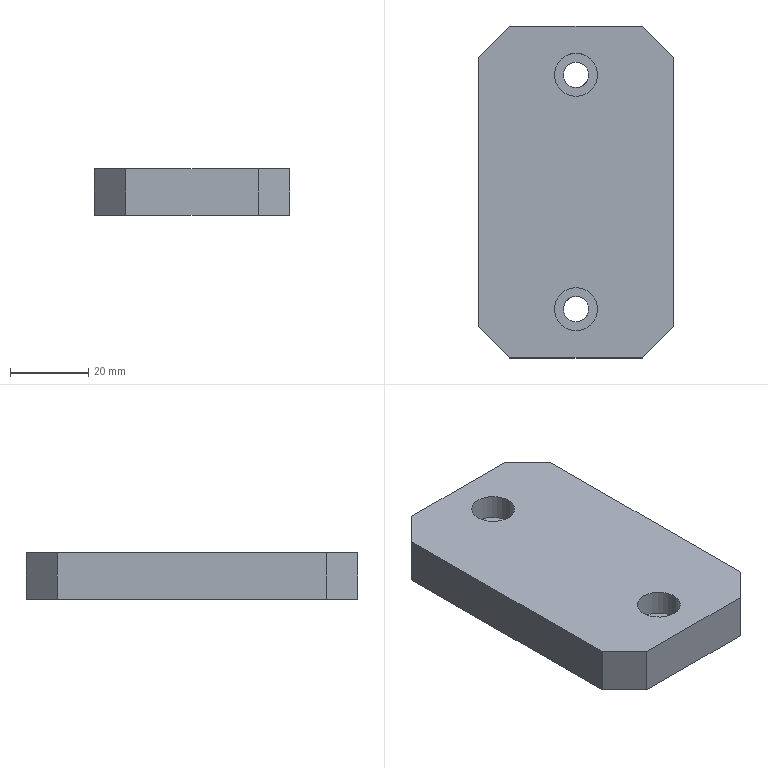Part | STEP file | P011002NM02-000 | 1 solid | 16 faces | box 50 x 85 x 12 mm | volume 47864 mm3 | plane 12 | cylinder 4 | commonest cylinder face diameters 6.5 x2 11 x2
STEP:
#1=CARTESIAN_POINT('',(0.,0.,0.));
#2=DIRECTION('',(0.,0.,1.));
#3=DIRECTION('',(1.,0.,0.));
#4=AXIS2_PLACEMENT_3D('',#1,#2,#3);
#5=CARTESIAN_POINT('',(227.,150.,9.));
#6=VERTEX_POINT('',#5);
#7=CARTESIAN_POINT('',(193.,150.,9.));
#8=VERTEX_POINT('',#7);
#9=CARTESIAN_POINT('',(210.,150.,9.));
#10=DIRECTION('',(-1.,0.,0.));
#11=VECTOR('',#10,1.);
#12=LINE('',#9,#11);
#13=CARTESIAN_POINT('',(210.,150.,6.));
#14=DIRECTION('',(0.,-1.,0.));
#15=DIRECTION('',(0.,0.,1.));
#16=AXIS2_PLACEMENT_3D('',#13,#14,#15);
#17=PLANE('',#16);
#18=CARTESIAN_POINT('',(3.,0.));
#19=DIRECTION('',(0.,1.));
#20=VECTOR('',#19,1.);
#21=LINE('',#18,#20);
#22=(GEOMETRIC_REPRESENTATION_CONTEXT(2)PARAMETRIC_REPRESENTATION_CONTEXT()REPRESENTATION_CONTEXT('',''));
#23=DEFINITIONAL_REPRESENTATION('',(#21),#22);
#24=PCURVE('',#17,#23);
#25=CARTESIAN_POINT('',(178.,-325.,9.));
#26=DIRECTION('',(0.,0.,1.));
#27=DIRECTION('',(1.,0.,0.));
#28=AXIS2_PLACEMENT_3D('',#25,#26,#27);
#29=PLANE('',#28);
#30=CARTESIAN_POINT('',(32.,475.));
#31=DIRECTION('',(-1.,0.));
#32=VECTOR('',#31,1.);
#33=LINE('',#30,#32);
#34=(GEOMETRIC_REPRESENTATION_CONTEXT(2)PARAMETRIC_REPRESENTATION_CONTEXT()REPRESENTATION_CONTEXT('',''));
#35=DEFINITIONAL_REPRESENTATION('',(#33),#34);
#36=PCURVE('',#29,#35);
#37=SURFACE_CURVE('',#12,(#24,#36),.PCURVE_S1.);
#38=EDGE_CURVE('',#6,#8,#37,.T.);
#39=ORIENTED_EDGE('',*,*,#38,.F.);
#40=CARTESIAN_POINT('',(227.,150.,21.));
#41=VERTEX_POINT('',#40);
#42=CARTESIAN_POINT('',(227.,150.,6.));
#43=DIRECTION('',(0.,0.,1.));
#44=VECTOR('',#43,1.);
#45=LINE('',#42,#44);
#46=CARTESIAN_POINT('',(0.,-17.));
#47=DIRECTION('',(1.,0.));
#48=VECTOR('',#47,1.);
#49=LINE('',#46,#48);
#50=(GEOMETRIC_REPRESENTATION_CONTEXT(2)PARAMETRIC_REPRESENTATION_CONTEXT()REPRESENTATION_CONTEXT('',''));
#51=DEFINITIONAL_REPRESENTATION('',(#49),#50);
#52=PCURVE('',#17,#51);
#53=CARTESIAN_POINT('',(235.,158.,6.));
#54=DIRECTION('',(-0.7071,0.7071,0.));
#55=DIRECTION('',(-0.7071,-0.7071,0.));
#56=AXIS2_PLACEMENT_3D('',#53,#54,#55);
#57=PLANE('',#56);
#58=CARTESIAN_POINT('',(11.314,0.));
#59=DIRECTION('',(0.,1.));
#60=VECTOR('',#59,1.);
#61=LINE('',#58,#60);
#62=(GEOMETRIC_REPRESENTATION_CONTEXT(2)PARAMETRIC_REPRESENTATION_CONTEXT()REPRESENTATION_CONTEXT('',''));
#63=DEFINITIONAL_REPRESENTATION('',(#61),#62);
#64=PCURVE('',#57,#63);
#65=SURFACE_CURVE('',#45,(#52,#64),.PCURVE_S1.);
#66=EDGE_CURVE('',#6,#41,#65,.T.);
#67=ORIENTED_EDGE('',*,*,#66,.T.);
#68=CARTESIAN_POINT('',(193.,150.,21.));
#69=VERTEX_POINT('',#68);
#70=CARTESIAN_POINT('',(210.,150.,21.));
#71=DIRECTION('',(-1.,0.,0.));
#72=VECTOR('',#71,1.);
#73=LINE('',#70,#72);
#74=CARTESIAN_POINT('',(15.,0.));
#75=DIRECTION('',(0.,1.));
#76=VECTOR('',#75,1.);
#77=LINE('',#74,#76);
#78=(GEOMETRIC_REPRESENTATION_CONTEXT(2)PARAMETRIC_REPRESENTATION_CONTEXT()REPRESENTATION_CONTEXT('',''));
#79=DEFINITIONAL_REPRESENTATION('',(#77),#78);
#80=PCURVE('',#17,#79);
#81=CARTESIAN_POINT('',(217.5,195.,21.));
#82=DIRECTION('',(0.,0.,1.));
#83=DIRECTION('',(1.,0.,0.));
#84=AXIS2_PLACEMENT_3D('',#81,#82,#83);
#85=PLANE('',#84);
#86=CARTESIAN_POINT('',(-7.5,-45.));
#87=DIRECTION('',(-1.,0.));
#88=VECTOR('',#87,1.);
#89=LINE('',#86,#88);
#90=(GEOMETRIC_REPRESENTATION_CONTEXT(2)PARAMETRIC_REPRESENTATION_CONTEXT()REPRESENTATION_CONTEXT('',''));
#91=DEFINITIONAL_REPRESENTATION('',(#89),#90);
#92=PCURVE('',#85,#91);
#93=SURFACE_CURVE('',#73,(#80,#92),.PCURVE_S1.);
#94=EDGE_CURVE('',#41,#69,#93,.T.);
#95=ORIENTED_EDGE('',*,*,#94,.T.);
#96=CARTESIAN_POINT('',(193.,150.,6.));
#97=DIRECTION('',(0.,0.,-1.));
#98=VECTOR('',#97,1.);
#99=LINE('',#96,#98);
#100=CARTESIAN_POINT('',(0.,17.));
#101=DIRECTION('',(-1.,0.));
#102=VECTOR('',#101,1.);
#103=LINE('',#100,#102);
#104=(GEOMETRIC_REPRESENTATION_CONTEXT(2)PARAMETRIC_REPRESENTATION_CONTEXT()REPRESENTATION_CONTEXT('',''));
#105=DEFINITIONAL_REPRESENTATION('',(#103),#104);
#106=PCURVE('',#17,#105);
#107=CARTESIAN_POINT('',(193.,150.,6.));
#108=DIRECTION('',(0.7071,0.7071,0.));
#109=DIRECTION('',(-0.7071,0.7071,0.));
#110=AXIS2_PLACEMENT_3D('',#107,#108,#109);
#111=PLANE('',#110);
#112=CARTESIAN_POINT('',(0.,0.));
#113=DIRECTION('',(0.,-1.));
#114=VECTOR('',#113,1.);
#115=LINE('',#112,#114);
#116=(GEOMETRIC_REPRESENTATION_CONTEXT(2)PARAMETRIC_REPRESENTATION_CONTEXT()REPRESENTATION_CONTEXT('',''));
#117=DEFINITIONAL_REPRESENTATION('',(#115),#116);
#118=PCURVE('',#111,#117);
#119=SURFACE_CURVE('',#99,(#106,#118),.PCURVE_S1.);
#120=EDGE_CURVE('',#69,#8,#119,.T.);
#121=ORIENTED_EDGE('',*,*,#120,.T.);
#122=EDGE_LOOP('',(#39,#67,#95,#121));
#123=FACE_BOUND('',#122,.T.);
#124=ADVANCED_FACE('',(#123),#17,.T.);
#125=CARTESIAN_POINT('',(235.,227.,9.));
#126=VERTEX_POINT('',#125);
#127=CARTESIAN_POINT('',(235.,158.,9.));
#128=VERTEX_POINT('',#127);
#129=CARTESIAN_POINT('',(235.,192.5,9.));
#130=DIRECTION('',(0.,-1.,0.));
#131=VECTOR('',#130,1.);
#132=LINE('',#129,#131);
#133=CARTESIAN_POINT('',(235.,192.5,6.));
#134=DIRECTION('',(1.,0.,0.));
#135=DIRECTION('',(0.,0.,-1.));
#136=AXIS2_PLACEMENT_3D('',#133,#134,#135);
#137=PLANE('',#136);
#138=CARTESIAN_POINT('',(-3.,0.));
#139=DIRECTION('',(0.,-1.));
#140=VECTOR('',#139,1.);
#141=LINE('',#138,#140);
#142=(GEOMETRIC_REPRESENTATION_CONTEXT(2)PARAMETRIC_REPRESENTATION_CONTEXT()REPRESENTATION_CONTEXT('',''));
#143=DEFINITIONAL_REPRESENTATION('',(#141),#142);
#144=PCURVE('',#137,#143);
#145=CARTESIAN_POINT('',(57.,517.5));
#146=DIRECTION('',(0.,-1.));
#147=VECTOR('',#146,1.);
#148=LINE('',#145,#147);
#149=(GEOMETRIC_REPRESENTATION_CONTEXT(2)PARAMETRIC_REPRESENTATION_CONTEXT()REPRESENTATION_CONTEXT('',''));
#150=DEFINITIONAL_REPRESENTATION('',(#148),#149);
#151=PCURVE('',#29,#150);
#152=SURFACE_CURVE('',#132,(#144,#151),.PCURVE_S1.);
#153=EDGE_CURVE('',#126,#128,#152,.T.);
#154=ORIENTED_EDGE('',*,*,#153,.F.);
#155=CARTESIAN_POINT('',(235.,227.,21.));
#156=VERTEX_POINT('',#155);
#157=CARTESIAN_POINT('',(235.,227.,6.));
#158=DIRECTION('',(0.,0.,1.));
#159=VECTOR('',#158,1.);
#160=LINE('',#157,#159);
#161=CARTESIAN_POINT('',(0.,34.5));
#162=DIRECTION('',(-1.,0.));
#163=VECTOR('',#162,1.);
#164=LINE('',#161,#163);
#165=(GEOMETRIC_REPRESENTATION_CONTEXT(2)PARAMETRIC_REPRESENTATION_CONTEXT()REPRESENTATION_CONTEXT('',''));
#166=DEFINITIONAL_REPRESENTATION('',(#164),#165);
#167=PCURVE('',#137,#166);
#168=CARTESIAN_POINT('',(227.,235.,6.));
#169=DIRECTION('',(-0.7071,-0.7071,0.));
#170=DIRECTION('',(0.7071,-0.7071,0.));
#171=AXIS2_PLACEMENT_3D('',#168,#169,#170);
#172=PLANE('',#171);
#173=CARTESIAN_POINT('',(11.314,0.));
#174=DIRECTION('',(0.,1.));
#175=VECTOR('',#174,1.);
#176=LINE('',#173,#175);
#177=(GEOMETRIC_REPRESENTATION_CONTEXT(2)PARAMETRIC_REPRESENTATION_CONTEXT()REPRESENTATION_CONTEXT('',''));
#178=DEFINITIONAL_REPRESENTATION('',(#176),#177);
#179=PCURVE('',#172,#178);
#180=SURFACE_CURVE('',#160,(#167,#179),.PCURVE_S1.);
#181=EDGE_CURVE('',#126,#156,#180,.T.);
#182=ORIENTED_EDGE('',*,*,#181,.T.);
#183=CARTESIAN_POINT('',(235.,158.,21.));
#184=VERTEX_POINT('',#183);
#185=CARTESIAN_POINT('',(235.,192.5,21.));
#186=DIRECTION('',(0.,-1.,0.));
#187=VECTOR('',#186,1.);
#188=LINE('',#185,#187);
#189=CARTESIAN_POINT('',(-15.,0.));
#190=DIRECTION('',(0.,-1.));
#191=VECTOR('',#190,1.);
#192=LINE('',#189,#191);
#193=(GEOMETRIC_REPRESENTATION_CONTEXT(2)PARAMETRIC_REPRESENTATION_CONTEXT()REPRESENTATION_CONTEXT('',''));
#194=DEFINITIONAL_REPRESENTATION('',(#192),#193);
#195=PCURVE('',#137,#194);
#196=CARTESIAN_POINT('',(17.5,-2.5));
#197=DIRECTION('',(0.,-1.));
#198=VECTOR('',#197,1.);
#199=LINE('',#196,#198);
#200=(GEOMETRIC_REPRESENTATION_CONTEXT(2)PARAMETRIC_REPRESENTATION_CONTEXT()REPRESENTATION_CONTEXT('',''));
#201=DEFINITIONAL_REPRESENTATION('',(#199),#200);
#202=PCURVE('',#85,#201);
#203=SURFACE_CURVE('',#188,(#195,#202),.PCURVE_S1.);
#204=EDGE_CURVE('',#156,#184,#203,.T.);
#205=ORIENTED_EDGE('',*,*,#204,.T.);
#206=CARTESIAN_POINT('',(235.,158.,6.));
#207=DIRECTION('',(0.,0.,-1.));
#208=VECTOR('',#207,1.);
#209=LINE('',#206,#208);
#210=CARTESIAN_POINT('',(0.,-34.5));
#211=DIRECTION('',(1.,0.));
#212=VECTOR('',#211,1.);
#213=LINE('',#210,#212);
#214=(GEOMETRIC_REPRESENTATION_CONTEXT(2)PARAMETRIC_REPRESENTATION_CONTEXT()REPRESENTATION_CONTEXT('',''));
#215=DEFINITIONAL_REPRESENTATION('',(#213),#214);
#216=PCURVE('',#137,#215);
#217=CARTESIAN_POINT('',(0.,0.));
#218=DIRECTION('',(0.,-1.));
#219=VECTOR('',#218,1.);
#220=LINE('',#217,#219);
#221=(GEOMETRIC_REPRESENTATION_CONTEXT(2)PARAMETRIC_REPRESENTATION_CONTEXT()REPRESENTATION_CONTEXT('',''));
#222=DEFINITIONAL_REPRESENTATION('',(#220),#221);
#223=PCURVE('',#57,#222);
#224=SURFACE_CURVE('',#209,(#216,#223),.PCURVE_S1.);
#225=EDGE_CURVE('',#184,#128,#224,.T.);
#226=ORIENTED_EDGE('',*,*,#225,.T.);
#227=EDGE_LOOP('',(#154,#182,#205,#226));
#228=FACE_BOUND('',#227,.T.);
#229=ADVANCED_FACE('',(#228),#137,.T.);
#230=CARTESIAN_POINT('',(193.,235.,9.));
#231=VERTEX_POINT('',#230);
#232=CARTESIAN_POINT('',(227.,235.,9.));
#233=VERTEX_POINT('',#232);
#234=CARTESIAN_POINT('',(210.,235.,9.));
#235=DIRECTION('',(1.,0.,0.));
#236=VECTOR('',#235,1.);
#237=LINE('',#234,#236);
#238=CARTESIAN_POINT('',(210.,235.,6.));
#239=DIRECTION('',(0.,1.,0.));
#240=DIRECTION('',(0.,0.,-1.));
#241=AXIS2_PLACEMENT_3D('',#238,#239,#240);
#242=PLANE('',#241);
#243=CARTESIAN_POINT('',(-3.,0.));
#244=DIRECTION('',(0.,-1.));
#245=VECTOR('',#244,1.);
#246=LINE('',#243,#245);
#247=(GEOMETRIC_REPRESENTATION_CONTEXT(2)PARAMETRIC_REPRESENTATION_CONTEXT()REPRESENTATION_CONTEXT('',''));
#248=DEFINITIONAL_REPRESENTATION('',(#246),#247);
#249=PCURVE('',#242,#248);
#250=CARTESIAN_POINT('',(32.,560.));
#251=DIRECTION('',(1.,0.));
#252=VECTOR('',#251,1.);
#253=LINE('',#250,#252);
#254=(GEOMETRIC_REPRESENTATION_CONTEXT(2)PARAMETRIC_REPRESENTATION_CONTEXT()REPRESENTATION_CONTEXT('',''));
#255=DEFINITIONAL_REPRESENTATION('',(#253),#254);
#256=PCURVE('',#29,#255);
#257=SURFACE_CURVE('',#237,(#249,#256),.PCURVE_S1.);
#258=EDGE_CURVE('',#231,#233,#257,.T.);
#259=ORIENTED_EDGE('',*,*,#258,.F.);
#260=CARTESIAN_POINT('',(193.,235.,21.));
#261=VERTEX_POINT('',#260);
#262=CARTESIAN_POINT('',(193.,235.,6.));
#263=DIRECTION('',(0.,0.,1.));
#264=VECTOR('',#263,1.);
#265=LINE('',#262,#264);
#266=CARTESIAN_POINT('',(0.,17.));
#267=DIRECTION('',(-1.,0.));
#268=VECTOR('',#267,1.);
#269=LINE('',#266,#268);
#270=(GEOMETRIC_REPRESENTATION_CONTEXT(2)PARAMETRIC_REPRESENTATION_CONTEXT()REPRESENTATION_CONTEXT('',''));
#271=DEFINITIONAL_REPRESENTATION('',(#269),#270);
#272=PCURVE('',#242,#271);
#273=CARTESIAN_POINT('',(185.,227.,6.));
#274=DIRECTION('',(0.7071,-0.7071,0.));
#275=DIRECTION('',(0.7071,0.7071,0.));
#276=AXIS2_PLACEMENT_3D('',#273,#274,#275);
#277=PLANE('',#276);
#278=CARTESIAN_POINT('',(11.314,0.));
#279=DIRECTION('',(0.,1.));
#280=VECTOR('',#279,1.);
#281=LINE('',#278,#280);
#282=(GEOMETRIC_REPRESENTATION_CONTEXT(2)PARAMETRIC_REPRESENTATION_CONTEXT()REPRESENTATION_CONTEXT('',''));
#283=DEFINITIONAL_REPRESENTATION('',(#281),#282);
#284=PCURVE('',#277,#283);
#285=SURFACE_CURVE('',#265,(#272,#284),.PCURVE_S1.);
#286=EDGE_CURVE('',#231,#261,#285,.T.);
#287=ORIENTED_EDGE('',*,*,#286,.T.);
#288=CARTESIAN_POINT('',(227.,235.,21.));
#289=VERTEX_POINT('',#288);
#290=CARTESIAN_POINT('',(210.,235.,21.));
#291=DIRECTION('',(1.,0.,0.));
#292=VECTOR('',#291,1.);
#293=LINE('',#290,#292);
#294=CARTESIAN_POINT('',(-15.,0.));
#295=DIRECTION('',(0.,-1.));
#296=VECTOR('',#295,1.);
#297=LINE('',#294,#296);
#298=(GEOMETRIC_REPRESENTATION_CONTEXT(2)PARAMETRIC_REPRESENTATION_CONTEXT()REPRESENTATION_CONTEXT('',''));
#299=DEFINITIONAL_REPRESENTATION('',(#297),#298);
#300=PCURVE('',#242,#299);
#301=CARTESIAN_POINT('',(-7.5,40.));
#302=DIRECTION('',(1.,0.));
#303=VECTOR('',#302,1.);
#304=LINE('',#301,#303);
#305=(GEOMETRIC_REPRESENTATION_CONTEXT(2)PARAMETRIC_REPRESENTATION_CONTEXT()REPRESENTATION_CONTEXT('',''));
#306=DEFINITIONAL_REPRESENTATION('',(#304),#305);
#307=PCURVE('',#85,#306);
#308=SURFACE_CURVE('',#293,(#300,#307),.PCURVE_S1.);
#309=EDGE_CURVE('',#261,#289,#308,.T.);
#310=ORIENTED_EDGE('',*,*,#309,.T.);
#311=CARTESIAN_POINT('',(227.,235.,6.));
#312=DIRECTION('',(0.,0.,-1.));
#313=VECTOR('',#312,1.);
#314=LINE('',#311,#313);
#315=CARTESIAN_POINT('',(0.,-17.));
#316=DIRECTION('',(1.,0.));
#317=VECTOR('',#316,1.);
#318=LINE('',#315,#317);
#319=(GEOMETRIC_REPRESENTATION_CONTEXT(2)PARAMETRIC_REPRESENTATION_CONTEXT()REPRESENTATION_CONTEXT('',''));
#320=DEFINITIONAL_REPRESENTATION('',(#318),#319);
#321=PCURVE('',#242,#320);
#322=CARTESIAN_POINT('',(0.,0.));
#323=DIRECTION('',(0.,-1.));
#324=VECTOR('',#323,1.);
#325=LINE('',#322,#324);
#326=(GEOMETRIC_REPRESENTATION_CONTEXT(2)PARAMETRIC_REPRESENTATION_CONTEXT()REPRESENTATION_CONTEXT('',''));
#327=DEFINITIONAL_REPRESENTATION('',(#325),#326);
#328=PCURVE('',#172,#327);
#329=SURFACE_CURVE('',#314,(#321,#328),.PCURVE_S1.);
#330=EDGE_CURVE('',#289,#233,#329,.T.);
#331=ORIENTED_EDGE('',*,*,#330,.T.);
#332=EDGE_LOOP('',(#259,#287,#310,#331));
#333=FACE_BOUND('',#332,.T.);
#334=ADVANCED_FACE('',(#333),#242,.T.);
#335=CARTESIAN_POINT('',(210.,157.,21.));
#336=VERTEX_POINT('',#335);
#337=CARTESIAN_POINT('',(210.,162.5,21.));
#338=DIRECTION('',(0.,0.,1.));
#339=DIRECTION('',(0.,-1.,0.));
#340=AXIS2_PLACEMENT_3D('',#337,#338,#339);
#341=CIRCLE('',#340,5.5);
#342=CARTESIAN_POINT('',(-7.5,-32.5));
#343=DIRECTION('',(0.,-1.));
#344=AXIS2_PLACEMENT_2D('',#342,#343);
#345=CIRCLE('',#344,5.5);
#346=(GEOMETRIC_REPRESENTATION_CONTEXT(2)PARAMETRIC_REPRESENTATION_CONTEXT()REPRESENTATION_CONTEXT('',''));
#347=DEFINITIONAL_REPRESENTATION('',(#345),#346);
#348=PCURVE('',#85,#347);
#349=CARTESIAN_POINT('',(210.,162.5,22.));
#350=DIRECTION('',(0.,0.,1.));
#351=DIRECTION('',(0.,-1.,0.));
#352=AXIS2_PLACEMENT_3D('',#349,#350,#351);
#353=CYLINDRICAL_SURFACE('',#352,5.5);
#354=CARTESIAN_POINT('',(0.,-1.));
#355=DIRECTION('',(1.,0.));
#356=VECTOR('',#355,1.);
#357=LINE('',#354,#356);
#358=(GEOMETRIC_REPRESENTATION_CONTEXT(2)PARAMETRIC_REPRESENTATION_CONTEXT()REPRESENTATION_CONTEXT('',''));
#359=DEFINITIONAL_REPRESENTATION('',(#357),#358);
#360=PCURVE('',#353,#359);
#361=SURFACE_CURVE('',#341,(#348,#360),.PCURVE_S1.);
#362=EDGE_CURVE('',#336,#336,#361,.T.);
#363=ORIENTED_EDGE('',*,*,#362,.F.);
#364=EDGE_LOOP('',(#363));
#365=FACE_BOUND('',#364,.T.);
#366=CARTESIAN_POINT('',(210.,217.,21.));
#367=VERTEX_POINT('',#366);
#368=CARTESIAN_POINT('',(210.,222.5,21.));
#369=DIRECTION('',(0.,0.,1.));
#370=DIRECTION('',(0.,-1.,0.));
#371=AXIS2_PLACEMENT_3D('',#368,#369,#370);
#372=CIRCLE('',#371,5.5);
#373=CARTESIAN_POINT('',(-7.5,27.5));
#374=DIRECTION('',(0.,-1.));
#375=AXIS2_PLACEMENT_2D('',#373,#374);
#376=CIRCLE('',#375,5.5);
#377=(GEOMETRIC_REPRESENTATION_CONTEXT(2)PARAMETRIC_REPRESENTATION_CONTEXT()REPRESENTATION_CONTEXT('',''));
#378=DEFINITIONAL_REPRESENTATION('',(#376),#377);
#379=PCURVE('',#85,#378);
#380=CARTESIAN_POINT('',(210.,222.5,22.));
#381=DIRECTION('',(0.,0.,1.));
#382=DIRECTION('',(0.,-1.,0.));
#383=AXIS2_PLACEMENT_3D('',#380,#381,#382);
#384=CYLINDRICAL_SURFACE('',#383,5.5);
#385=CARTESIAN_POINT('',(0.,-1.));
#386=DIRECTION('',(1.,0.));
#387=VECTOR('',#386,1.);
#388=LINE('',#385,#387);
#389=(GEOMETRIC_REPRESENTATION_CONTEXT(2)PARAMETRIC_REPRESENTATION_CONTEXT()REPRESENTATION_CONTEXT('',''));
#390=DEFINITIONAL_REPRESENTATION('',(#388),#389);
#391=PCURVE('',#384,#390);
#392=SURFACE_CURVE('',#372,(#379,#391),.PCURVE_S1.);
#393=EDGE_CURVE('',#367,#367,#392,.T.);
#394=ORIENTED_EDGE('',*,*,#393,.F.);
#395=EDGE_LOOP('',(#394));
#396=FACE_BOUND('',#395,.T.);
#397=CARTESIAN_POINT('',(185.,158.,21.));
#398=VERTEX_POINT('',#397);
#399=CARTESIAN_POINT('',(185.,227.,21.));
#400=VERTEX_POINT('',#399);
#401=CARTESIAN_POINT('',(185.,192.5,21.));
#402=DIRECTION('',(0.,1.,0.));
#403=VECTOR('',#402,1.);
#404=LINE('',#401,#403);
#405=CARTESIAN_POINT('',(-32.5,-2.5));
#406=DIRECTION('',(0.,1.));
#407=VECTOR('',#406,1.);
#408=LINE('',#405,#407);
#409=(GEOMETRIC_REPRESENTATION_CONTEXT(2)PARAMETRIC_REPRESENTATION_CONTEXT()REPRESENTATION_CONTEXT('',''));
#410=DEFINITIONAL_REPRESENTATION('',(#408),#409);
#411=PCURVE('',#85,#410);
#412=CARTESIAN_POINT('',(185.,192.5,6.));
#413=DIRECTION('',(-1.,0.,0.));
#414=DIRECTION('',(0.,0.,1.));
#415=AXIS2_PLACEMENT_3D('',#412,#413,#414);
#416=PLANE('',#415);
#417=CARTESIAN_POINT('',(15.,0.));
#418=DIRECTION('',(0.,1.));
#419=VECTOR('',#418,1.);
#420=LINE('',#417,#419);
#421=(GEOMETRIC_REPRESENTATION_CONTEXT(2)PARAMETRIC_REPRESENTATION_CONTEXT()REPRESENTATION_CONTEXT('',''));
#422=DEFINITIONAL_REPRESENTATION('',(#420),#421);
#423=PCURVE('',#416,#422);
#424=SURFACE_CURVE('',#404,(#411,#423),.PCURVE_S1.);
#425=EDGE_CURVE('',#398,#400,#424,.T.);
#426=ORIENTED_EDGE('',*,*,#425,.F.);
#427=CARTESIAN_POINT('',(182.75,160.25,21.));
#428=DIRECTION('',(0.7071,-0.7071,0.));
#429=VECTOR('',#428,1.);
#430=LINE('',#427,#429);
#431=CARTESIAN_POINT('',(-34.75,-34.75));
#432=DIRECTION('',(0.7071,-0.7071));
#433=VECTOR('',#432,1.);
#434=LINE('',#431,#433);
#435=(GEOMETRIC_REPRESENTATION_CONTEXT(2)PARAMETRIC_REPRESENTATION_CONTEXT()REPRESENTATION_CONTEXT('',''));
#436=DEFINITIONAL_REPRESENTATION('',(#434),#435);
#437=PCURVE('',#85,#436);
#438=CARTESIAN_POINT('',(14.496,15.));
#439=DIRECTION('',(-1.,0.));
#440=VECTOR('',#439,1.);
#441=LINE('',#438,#440);
#442=(GEOMETRIC_REPRESENTATION_CONTEXT(2)PARAMETRIC_REPRESENTATION_CONTEXT()REPRESENTATION_CONTEXT('',''));
#443=DEFINITIONAL_REPRESENTATION('',(#441),#442);
#444=PCURVE('',#111,#443);
#445=SURFACE_CURVE('',#430,(#437,#444),.PCURVE_S1.);
#446=EDGE_CURVE('',#398,#69,#445,.T.);
#447=ORIENTED_EDGE('',*,*,#446,.T.);
#448=ORIENTED_EDGE('',*,*,#94,.F.);
#449=CARTESIAN_POINT('',(244.75,167.75,21.));
#450=DIRECTION('',(0.7071,0.7071,0.));
#451=VECTOR('',#450,1.);
#452=LINE('',#449,#451);
#453=CARTESIAN_POINT('',(27.25,-27.25));
#454=DIRECTION('',(0.7071,0.7071));
#455=VECTOR('',#454,1.);
#456=LINE('',#453,#455);
#457=(GEOMETRIC_REPRESENTATION_CONTEXT(2)PARAMETRIC_REPRESENTATION_CONTEXT()REPRESENTATION_CONTEXT('',''));
#458=DEFINITIONAL_REPRESENTATION('',(#456),#457);
#459=PCURVE('',#85,#458);
#460=CARTESIAN_POINT('',(-13.789,15.));
#461=DIRECTION('',(-1.,0.));
#462=VECTOR('',#461,1.);
#463=LINE('',#460,#462);
#464=(GEOMETRIC_REPRESENTATION_CONTEXT(2)PARAMETRIC_REPRESENTATION_CONTEXT()REPRESENTATION_CONTEXT('',''));
#465=DEFINITIONAL_REPRESENTATION('',(#463),#464);
#466=PCURVE('',#57,#465);
#467=SURFACE_CURVE('',#452,(#459,#466),.PCURVE_S1.);
#468=EDGE_CURVE('',#41,#184,#467,.T.);
#469=ORIENTED_EDGE('',*,*,#468,.T.);
#470=ORIENTED_EDGE('',*,*,#204,.F.);
#471=CARTESIAN_POINT('',(242.25,219.75,21.));
#472=DIRECTION('',(-0.7071,0.7071,0.));
#473=VECTOR('',#472,1.);
#474=LINE('',#471,#473);
#475=CARTESIAN_POINT('',(24.75,24.75));
#476=DIRECTION('',(-0.7071,0.7071));
#477=VECTOR('',#476,1.);
#478=LINE('',#475,#477);
#479=(GEOMETRIC_REPRESENTATION_CONTEXT(2)PARAMETRIC_REPRESENTATION_CONTEXT()REPRESENTATION_CONTEXT('',''));
#480=DEFINITIONAL_REPRESENTATION('',(#478),#479);
#481=PCURVE('',#85,#480);
#482=CARTESIAN_POINT('',(21.567,15.));
#483=DIRECTION('',(-1.,0.));
#484=VECTOR('',#483,1.);
#485=LINE('',#482,#484);
#486=(GEOMETRIC_REPRESENTATION_CONTEXT(2)PARAMETRIC_REPRESENTATION_CONTEXT()REPRESENTATION_CONTEXT('',''));
#487=DEFINITIONAL_REPRESENTATION('',(#485),#486);
#488=PCURVE('',#172,#487);
#489=SURFACE_CURVE('',#474,(#481,#488),.PCURVE_S1.);
#490=EDGE_CURVE('',#156,#289,#489,.T.);
#491=ORIENTED_EDGE('',*,*,#490,.T.);
#492=ORIENTED_EDGE('',*,*,#309,.F.);
#493=CARTESIAN_POINT('',(185.25,227.25,21.));
#494=DIRECTION('',(-0.7071,-0.7071,0.));
#495=VECTOR('',#494,1.);
#496=LINE('',#493,#495);
#497=CARTESIAN_POINT('',(-32.25,32.25));
#498=DIRECTION('',(-0.7071,-0.7071));
#499=VECTOR('',#498,1.);
#500=LINE('',#497,#499);
#501=(GEOMETRIC_REPRESENTATION_CONTEXT(2)PARAMETRIC_REPRESENTATION_CONTEXT()REPRESENTATION_CONTEXT('',''));
#502=DEFINITIONAL_REPRESENTATION('',(#500),#501);
#503=PCURVE('',#85,#502);
#504=CARTESIAN_POINT('',(0.3536,15.));
#505=DIRECTION('',(-1.,0.));
#506=VECTOR('',#505,1.);
#507=LINE('',#504,#506);
#508=(GEOMETRIC_REPRESENTATION_CONTEXT(2)PARAMETRIC_REPRESENTATION_CONTEXT()REPRESENTATION_CONTEXT('',''));
#509=DEFINITIONAL_REPRESENTATION('',(#507),#508);
#510=PCURVE('',#277,#509);
#511=SURFACE_CURVE('',#496,(#503,#510),.PCURVE_S1.);
#512=EDGE_CURVE('',#261,#400,#511,.T.);
#513=ORIENTED_EDGE('',*,*,#512,.T.);
#514=EDGE_LOOP('',(#426,#447,#448,#469,#470,#491,#492,#513));
#515=FACE_BOUND('',#514,.T.);
#516=ADVANCED_FACE('',(#365,#396,#515),#85,.T.);
#517=CARTESIAN_POINT('',(185.,158.,9.));
#518=VERTEX_POINT('',#517);
#519=CARTESIAN_POINT('',(185.,227.,9.));
#520=VERTEX_POINT('',#519);
#521=CARTESIAN_POINT('',(185.,192.5,9.));
#522=DIRECTION('',(0.,1.,0.));
#523=VECTOR('',#522,1.);
#524=LINE('',#521,#523);
#525=CARTESIAN_POINT('',(3.,0.));
#526=DIRECTION('',(0.,1.));
#527=VECTOR('',#526,1.);
#528=LINE('',#525,#527);
#529=(GEOMETRIC_REPRESENTATION_CONTEXT(2)PARAMETRIC_REPRESENTATION_CONTEXT()REPRESENTATION_CONTEXT('',''));
#530=DEFINITIONAL_REPRESENTATION('',(#528),#529);
#531=PCURVE('',#416,#530);
#532=CARTESIAN_POINT('',(7.,517.5));
#533=DIRECTION('',(0.,1.));
#534=VECTOR('',#533,1.);
#535=LINE('',#532,#534);
#536=(GEOMETRIC_REPRESENTATION_CONTEXT(2)PARAMETRIC_REPRESENTATION_CONTEXT()REPRESENTATION_CONTEXT('',''));
#537=DEFINITIONAL_REPRESENTATION('',(#535),#536);
#538=PCURVE('',#29,#537);
#539=SURFACE_CURVE('',#524,(#531,#538),.PCURVE_S1.);
#540=EDGE_CURVE('',#518,#520,#539,.T.);
#541=ORIENTED_EDGE('',*,*,#540,.F.);
#542=CARTESIAN_POINT('',(185.,158.,6.));
#543=DIRECTION('',(0.,0.,1.));
#544=VECTOR('',#543,1.);
#545=LINE('',#542,#544);
#546=CARTESIAN_POINT('',(0.,-34.5));
#547=DIRECTION('',(1.,0.));
#548=VECTOR('',#547,1.);
#549=LINE('',#546,#548);
#550=(GEOMETRIC_REPRESENTATION_CONTEXT(2)PARAMETRIC_REPRESENTATION_CONTEXT()REPRESENTATION_CONTEXT('',''));
#551=DEFINITIONAL_REPRESENTATION('',(#549),#550);
#552=PCURVE('',#416,#551);
#553=CARTESIAN_POINT('',(11.314,0.));
#554=DIRECTION('',(0.,1.));
#555=VECTOR('',#554,1.);
#556=LINE('',#553,#555);
#557=(GEOMETRIC_REPRESENTATION_CONTEXT(2)PARAMETRIC_REPRESENTATION_CONTEXT()REPRESENTATION_CONTEXT('',''));
#558=DEFINITIONAL_REPRESENTATION('',(#556),#557);
#559=PCURVE('',#111,#558);
#560=SURFACE_CURVE('',#545,(#552,#559),.PCURVE_S1.);
#561=EDGE_CURVE('',#518,#398,#560,.T.);
#562=ORIENTED_EDGE('',*,*,#561,.T.);
#563=ORIENTED_EDGE('',*,*,#425,.T.);
#564=CARTESIAN_POINT('',(185.,227.,6.));
#565=DIRECTION('',(0.,0.,-1.));
#566=VECTOR('',#565,1.);
#567=LINE('',#564,#566);
#568=CARTESIAN_POINT('',(0.,34.5));
#569=DIRECTION('',(-1.,0.));
#570=VECTOR('',#569,1.);
#571=LINE('',#568,#570);
#572=(GEOMETRIC_REPRESENTATION_CONTEXT(2)PARAMETRIC_REPRESENTATION_CONTEXT()REPRESENTATION_CONTEXT('',''));
#573=DEFINITIONAL_REPRESENTATION('',(#571),#572);
#574=PCURVE('',#416,#573);
#575=CARTESIAN_POINT('',(0.,0.));
#576=DIRECTION('',(0.,-1.));
#577=VECTOR('',#576,1.);
#578=LINE('',#575,#577);
#579=(GEOMETRIC_REPRESENTATION_CONTEXT(2)PARAMETRIC_REPRESENTATION_CONTEXT()REPRESENTATION_CONTEXT('',''));
#580=DEFINITIONAL_REPRESENTATION('',(#578),#579);
#581=PCURVE('',#277,#580);
#582=SURFACE_CURVE('',#567,(#574,#581),.PCURVE_S1.);
#583=EDGE_CURVE('',#400,#520,#582,.T.);
#584=ORIENTED_EDGE('',*,*,#583,.T.);
#585=EDGE_LOOP('',(#541,#562,#563,#584));
#586=FACE_BOUND('',#585,.T.);
#587=ADVANCED_FACE('',(#586),#416,.T.);
#588=CARTESIAN_POINT('',(193.,150.,9.));
#589=DIRECTION('',(-0.7071,0.7071,0.));
#590=VECTOR('',#589,1.);
#591=LINE('',#588,#590);
#592=CARTESIAN_POINT('',(0.,3.));
#593=DIRECTION('',(1.,0.));
#594=VECTOR('',#593,1.);
#595=LINE('',#592,#594);
#596=(GEOMETRIC_REPRESENTATION_CONTEXT(2)PARAMETRIC_REPRESENTATION_CONTEXT()REPRESENTATION_CONTEXT('',''));
#597=DEFINITIONAL_REPRESENTATION('',(#595),#596);
#598=PCURVE('',#111,#597);
#599=CARTESIAN_POINT('',(15.,475.));
#600=DIRECTION('',(-0.7071,0.7071));
#601=VECTOR('',#600,1.);
#602=LINE('',#599,#601);
#603=(GEOMETRIC_REPRESENTATION_CONTEXT(2)PARAMETRIC_REPRESENTATION_CONTEXT()REPRESENTATION_CONTEXT('',''));
#604=DEFINITIONAL_REPRESENTATION('',(#602),#603);
#605=PCURVE('',#29,#604);
#606=SURFACE_CURVE('',#591,(#598,#605),.PCURVE_S1.);
#607=EDGE_CURVE('',#8,#518,#606,.T.);
#608=ORIENTED_EDGE('',*,*,#607,.F.);
#609=ORIENTED_EDGE('',*,*,#120,.F.);
#610=ORIENTED_EDGE('',*,*,#446,.F.);
#611=ORIENTED_EDGE('',*,*,#561,.F.);
#612=EDGE_LOOP('',(#608,#609,#610,#611));
#613=FACE_BOUND('',#612,.T.);
#614=ADVANCED_FACE('',(#613),#111,.F.);
#615=CARTESIAN_POINT('',(227.,235.,9.));
#616=DIRECTION('',(0.7071,-0.7071,0.));
#617=VECTOR('',#616,1.);
#618=LINE('',#615,#617);
#619=CARTESIAN_POINT('',(0.,3.));
#620=DIRECTION('',(1.,0.));
#621=VECTOR('',#620,1.);
#622=LINE('',#619,#621);
#623=(GEOMETRIC_REPRESENTATION_CONTEXT(2)PARAMETRIC_REPRESENTATION_CONTEXT()REPRESENTATION_CONTEXT('',''));
#624=DEFINITIONAL_REPRESENTATION('',(#622),#623);
#625=PCURVE('',#172,#624);
#626=CARTESIAN_POINT('',(49.,560.));
#627=DIRECTION('',(0.7071,-0.7071));
#628=VECTOR('',#627,1.);
#629=LINE('',#626,#628);
#630=(GEOMETRIC_REPRESENTATION_CONTEXT(2)PARAMETRIC_REPRESENTATION_CONTEXT()REPRESENTATION_CONTEXT('',''));
#631=DEFINITIONAL_REPRESENTATION('',(#629),#630);
#632=PCURVE('',#29,#631);
#633=SURFACE_CURVE('',#618,(#625,#632),.PCURVE_S1.);
#634=EDGE_CURVE('',#233,#126,#633,.T.);
#635=ORIENTED_EDGE('',*,*,#634,.F.);
#636=ORIENTED_EDGE('',*,*,#330,.F.);
#637=ORIENTED_EDGE('',*,*,#490,.F.);
#638=ORIENTED_EDGE('',*,*,#181,.F.);
#639=EDGE_LOOP('',(#635,#636,#637,#638));
#640=FACE_BOUND('',#639,.T.);
#641=ADVANCED_FACE('',(#640),#172,.F.);
#642=CARTESIAN_POINT('',(235.,158.,9.));
#643=DIRECTION('',(-0.7071,-0.7071,0.));
#644=VECTOR('',#643,1.);
#645=LINE('',#642,#644);
#646=CARTESIAN_POINT('',(0.,3.));
#647=DIRECTION('',(1.,0.));
#648=VECTOR('',#647,1.);
#649=LINE('',#646,#648);
#650=(GEOMETRIC_REPRESENTATION_CONTEXT(2)PARAMETRIC_REPRESENTATION_CONTEXT()REPRESENTATION_CONTEXT('',''));
#651=DEFINITIONAL_REPRESENTATION('',(#649),#650);
#652=PCURVE('',#57,#651);
#653=CARTESIAN_POINT('',(57.,483.));
#654=DIRECTION('',(-0.7071,-0.7071));
#655=VECTOR('',#654,1.);
#656=LINE('',#653,#655);
#657=(GEOMETRIC_REPRESENTATION_CONTEXT(2)PARAMETRIC_REPRESENTATION_CONTEXT()REPRESENTATION_CONTEXT('',''));
#658=DEFINITIONAL_REPRESENTATION('',(#656),#657);
#659=PCURVE('',#29,#658);
#660=SURFACE_CURVE('',#645,(#652,#659),.PCURVE_S1.);
#661=EDGE_CURVE('',#128,#6,#660,.T.);
#662=ORIENTED_EDGE('',*,*,#661,.F.);
#663=ORIENTED_EDGE('',*,*,#225,.F.);
#664=ORIENTED_EDGE('',*,*,#468,.F.);
#665=ORIENTED_EDGE('',*,*,#66,.F.);
#666=EDGE_LOOP('',(#662,#663,#664,#665));
#667=FACE_BOUND('',#666,.T.);
#668=ADVANCED_FACE('',(#667),#57,.F.);
#669=CARTESIAN_POINT('',(185.,227.,9.));
#670=DIRECTION('',(0.7071,0.7071,0.));
#671=VECTOR('',#670,1.);
#672=LINE('',#669,#671);
#673=CARTESIAN_POINT('',(0.,3.));
#674=DIRECTION('',(1.,0.));
#675=VECTOR('',#674,1.);
#676=LINE('',#673,#675);
#677=(GEOMETRIC_REPRESENTATION_CONTEXT(2)PARAMETRIC_REPRESENTATION_CONTEXT()REPRESENTATION_CONTEXT('',''));
#678=DEFINITIONAL_REPRESENTATION('',(#676),#677);
#679=PCURVE('',#277,#678);
#680=CARTESIAN_POINT('',(7.,552.));
#681=DIRECTION('',(0.7071,0.7071));
#682=VECTOR('',#681,1.);
#683=LINE('',#680,#682);
#684=(GEOMETRIC_REPRESENTATION_CONTEXT(2)PARAMETRIC_REPRESENTATION_CONTEXT()REPRESENTATION_CONTEXT('',''));
#685=DEFINITIONAL_REPRESENTATION('',(#683),#684);
#686=PCURVE('',#29,#685);
#687=SURFACE_CURVE('',#672,(#679,#686),.PCURVE_S1.);
#688=EDGE_CURVE('',#520,#231,#687,.T.);
#689=ORIENTED_EDGE('',*,*,#688,.F.);
#690=ORIENTED_EDGE('',*,*,#583,.F.);
#691=ORIENTED_EDGE('',*,*,#512,.F.);
#692=ORIENTED_EDGE('',*,*,#286,.F.);
#693=EDGE_LOOP('',(#689,#690,#691,#692));
#694=FACE_BOUND('',#693,.T.);
#695=ADVANCED_FACE('',(#694),#277,.F.);
#696=CARTESIAN_POINT('',(213.25,162.5,9.));
#697=VERTEX_POINT('',#696);
#698=CARTESIAN_POINT('',(210.,159.25,9.));
#699=VERTEX_POINT('',#698);
#700=CARTESIAN_POINT('',(210.,162.5,9.));
#701=DIRECTION('',(0.,0.,1.));
#702=DIRECTION('',(1.,0.,0.));
#703=AXIS2_PLACEMENT_3D('',#700,#701,#702);
#704=CIRCLE('',#703,3.25);
#705=CARTESIAN_POINT('',(32.,487.5));
#706=DIRECTION('',(1.,0.));
#707=AXIS2_PLACEMENT_2D('',#705,#706);
#708=CIRCLE('',#707,3.25);
#709=(GEOMETRIC_REPRESENTATION_CONTEXT(2)PARAMETRIC_REPRESENTATION_CONTEXT()REPRESENTATION_CONTEXT('',''));
#710=DEFINITIONAL_REPRESENTATION('',(#708),#709);
#711=PCURVE('',#29,#710);
#712=CARTESIAN_POINT('',(210.,162.5,22.));
#713=DIRECTION('',(0.,0.,1.));
#714=DIRECTION('',(0.,-1.,0.));
#715=AXIS2_PLACEMENT_3D('',#712,#713,#714);
#716=CYLINDRICAL_SURFACE('',#715,3.25);
#717=CARTESIAN_POINT('',(1.571,-13.));
#718=DIRECTION('',(1.,0.));
#719=VECTOR('',#718,1.);
#720=LINE('',#717,#719);
#721=(GEOMETRIC_REPRESENTATION_CONTEXT(2)PARAMETRIC_REPRESENTATION_CONTEXT()REPRESENTATION_CONTEXT('',''));
#722=DEFINITIONAL_REPRESENTATION('',(#720),#721);
#723=PCURVE('',#716,#722);
#724=SURFACE_CURVE('',#704,(#711,#723),.PCURVE_S1.);
#725=EDGE_CURVE('',#697,#699,#724,.T.);
#726=ORIENTED_EDGE('',*,*,#725,.T.);
#727=CARTESIAN_POINT('',(210.,162.5,9.));
#728=DIRECTION('',(0.,0.,1.));
#729=DIRECTION('',(1.,0.,0.));
#730=AXIS2_PLACEMENT_3D('',#727,#728,#729);
#731=CIRCLE('',#730,3.25);
#732=CARTESIAN_POINT('',(32.,487.5));
#733=DIRECTION('',(1.,0.));
#734=AXIS2_PLACEMENT_2D('',#732,#733);
#735=CIRCLE('',#734,3.25);
#736=(GEOMETRIC_REPRESENTATION_CONTEXT(2)PARAMETRIC_REPRESENTATION_CONTEXT()REPRESENTATION_CONTEXT('',''));
#737=DEFINITIONAL_REPRESENTATION('',(#735),#736);
#738=PCURVE('',#29,#737);
#739=CARTESIAN_POINT('',(-4.712,-13.));
#740=DIRECTION('',(1.,0.));
#741=VECTOR('',#740,1.);
#742=LINE('',#739,#741);
#743=(GEOMETRIC_REPRESENTATION_CONTEXT(2)PARAMETRIC_REPRESENTATION_CONTEXT()REPRESENTATION_CONTEXT('',''));
#744=DEFINITIONAL_REPRESENTATION('',(#742),#743);
#745=PCURVE('',#716,#744);
#746=SURFACE_CURVE('',#731,(#738,#745),.PCURVE_S1.);
#747=EDGE_CURVE('',#699,#697,#746,.T.);
#748=ORIENTED_EDGE('',*,*,#747,.T.);
#749=EDGE_LOOP('',(#726,#748));
#750=FACE_BOUND('',#749,.T.);
#751=CARTESIAN_POINT('',(213.25,222.5,9.));
#752=VERTEX_POINT('',#751);
#753=CARTESIAN_POINT('',(210.,219.25,9.));
#754=VERTEX_POINT('',#753);
#755=CARTESIAN_POINT('',(210.,222.5,9.));
#756=DIRECTION('',(0.,0.,1.));
#757=DIRECTION('',(1.,0.,0.));
#758=AXIS2_PLACEMENT_3D('',#755,#756,#757);
#759=CIRCLE('',#758,3.25);
#760=CARTESIAN_POINT('',(32.,547.5));
#761=DIRECTION('',(1.,0.));
#762=AXIS2_PLACEMENT_2D('',#760,#761);
#763=CIRCLE('',#762,3.25);
#764=(GEOMETRIC_REPRESENTATION_CONTEXT(2)PARAMETRIC_REPRESENTATION_CONTEXT()REPRESENTATION_CONTEXT('',''));
#765=DEFINITIONAL_REPRESENTATION('',(#763),#764);
#766=PCURVE('',#29,#765);
#767=CARTESIAN_POINT('',(210.,222.5,22.));
#768=DIRECTION('',(0.,0.,1.));
#769=DIRECTION('',(0.,-1.,0.));
#770=AXIS2_PLACEMENT_3D('',#767,#768,#769);
#771=CYLINDRICAL_SURFACE('',#770,3.25);
#772=CARTESIAN_POINT('',(1.571,-13.));
#773=DIRECTION('',(1.,0.));
#774=VECTOR('',#773,1.);
#775=LINE('',#772,#774);
#776=(GEOMETRIC_REPRESENTATION_CONTEXT(2)PARAMETRIC_REPRESENTATION_CONTEXT()REPRESENTATION_CONTEXT('',''));
#777=DEFINITIONAL_REPRESENTATION('',(#775),#776);
#778=PCURVE('',#771,#777);
#779=SURFACE_CURVE('',#759,(#766,#778),.PCURVE_S1.);
#780=EDGE_CURVE('',#752,#754,#779,.T.);
#781=ORIENTED_EDGE('',*,*,#780,.T.);
#782=CARTESIAN_POINT('',(210.,222.5,9.));
#783=DIRECTION('',(0.,0.,1.));
#784=DIRECTION('',(1.,0.,0.));
#785=AXIS2_PLACEMENT_3D('',#782,#783,#784);
#786=CIRCLE('',#785,3.25);
#787=CARTESIAN_POINT('',(32.,547.5));
#788=DIRECTION('',(1.,0.));
#789=AXIS2_PLACEMENT_2D('',#787,#788);
#790=CIRCLE('',#789,3.25);
#791=(GEOMETRIC_REPRESENTATION_CONTEXT(2)PARAMETRIC_REPRESENTATION_CONTEXT()REPRESENTATION_CONTEXT('',''));
#792=DEFINITIONAL_REPRESENTATION('',(#790),#791);
#793=PCURVE('',#29,#792);
#794=CARTESIAN_POINT('',(-4.712,-13.));
#795=DIRECTION('',(1.,0.));
#796=VECTOR('',#795,1.);
#797=LINE('',#794,#796);
#798=(GEOMETRIC_REPRESENTATION_CONTEXT(2)PARAMETRIC_REPRESENTATION_CONTEXT()REPRESENTATION_CONTEXT('',''));
#799=DEFINITIONAL_REPRESENTATION('',(#797),#798);
#800=PCURVE('',#771,#799);
#801=SURFACE_CURVE('',#786,(#793,#800),.PCURVE_S1.);
#802=EDGE_CURVE('',#754,#752,#801,.T.);
#803=ORIENTED_EDGE('',*,*,#802,.T.);
#804=EDGE_LOOP('',(#781,#803));
#805=FACE_BOUND('',#804,.T.);
#806=ORIENTED_EDGE('',*,*,#661,.T.);
#807=ORIENTED_EDGE('',*,*,#38,.T.);
#808=ORIENTED_EDGE('',*,*,#607,.T.);
#809=ORIENTED_EDGE('',*,*,#540,.T.);
#810=ORIENTED_EDGE('',*,*,#688,.T.);
#811=ORIENTED_EDGE('',*,*,#258,.T.);
#812=ORIENTED_EDGE('',*,*,#634,.T.);
#813=ORIENTED_EDGE('',*,*,#153,.T.);
#814=EDGE_LOOP('',(#806,#807,#808,#809,#810,#811,#812,#813));
#815=FACE_BOUND('',#814,.T.);
#816=ADVANCED_FACE('',(#750,#805,#815),#29,.F.);
#817=CARTESIAN_POINT('',(210.,219.25,14.5));
#818=VERTEX_POINT('',#817);
#819=CARTESIAN_POINT('',(210.,222.5,14.5));
#820=DIRECTION('',(0.,0.,1.));
#821=DIRECTION('',(0.,-1.,0.));
#822=AXIS2_PLACEMENT_3D('',#819,#820,#821);
#823=CIRCLE('',#822,3.25);
#824=CARTESIAN_POINT('',(0.,-7.5));
#825=DIRECTION('',(1.,0.));
#826=VECTOR('',#825,1.);
#827=LINE('',#824,#826);
#828=(GEOMETRIC_REPRESENTATION_CONTEXT(2)PARAMETRIC_REPRESENTATION_CONTEXT()REPRESENTATION_CONTEXT('',''));
#829=DEFINITIONAL_REPRESENTATION('',(#827),#828);
#830=PCURVE('',#771,#829);
#831=CARTESIAN_POINT('',(210.,222.5,14.5));
#832=DIRECTION('',(0.,0.,1.));
#833=DIRECTION('',(0.,-1.,0.));
#834=AXIS2_PLACEMENT_3D('',#831,#832,#833);
#835=PLANE('',#834);
#836=CARTESIAN_POINT('',(0.,0.));
#837=DIRECTION('',(1.,0.));
#838=AXIS2_PLACEMENT_2D('',#836,#837);
#839=CIRCLE('',#838,3.25);
#840=(GEOMETRIC_REPRESENTATION_CONTEXT(2)PARAMETRIC_REPRESENTATION_CONTEXT()REPRESENTATION_CONTEXT('',''));
#841=DEFINITIONAL_REPRESENTATION('',(#839),#840);
#842=PCURVE('',#835,#841);
#843=SURFACE_CURVE('',#823,(#830,#842),.PCURVE_S1.);
#844=EDGE_CURVE('',#818,#818,#843,.T.);
#845=ORIENTED_EDGE('',*,*,#844,.F.);
#846=CARTESIAN_POINT('',(210.,219.25,9.));
#847=CARTESIAN_POINT('',(210.,219.25,14.5));
#848=B_SPLINE_CURVE_WITH_KNOTS('',1,(#846,#847),.UNSPECIFIED.,.F.,.F.,(2,2),(-13.,-7.5),.PIECEWISE_BEZIER_KNOTS.);
#849=CARTESIAN_POINT('',(0.,0.));
#850=DIRECTION('',(0.,1.));
#851=VECTOR('',#850,1.);
#852=LINE('',#849,#851);
#853=(GEOMETRIC_REPRESENTATION_CONTEXT(2)PARAMETRIC_REPRESENTATION_CONTEXT()REPRESENTATION_CONTEXT('',''));
#854=DEFINITIONAL_REPRESENTATION('',(#852),#853);
#855=PCURVE('',#771,#854);
#856=CARTESIAN_POINT('',(6.283,0.));
#857=DIRECTION('',(0.,1.));
#858=VECTOR('',#857,1.);
#859=LINE('',#856,#858);
#860=(GEOMETRIC_REPRESENTATION_CONTEXT(2)PARAMETRIC_REPRESENTATION_CONTEXT()REPRESENTATION_CONTEXT('',''));
#861=DEFINITIONAL_REPRESENTATION('',(#859),#860);
#862=PCURVE('',#771,#861);
#863=SEAM_CURVE('',#848,(#855,#862),.PCURVE_S1.);
#864=EDGE_CURVE('',#754,#818,#863,.T.);
#865=ORIENTED_EDGE('',*,*,#864,.F.);
#866=ORIENTED_EDGE('',*,*,#802,.T.);
#867=ORIENTED_EDGE('',*,*,#780,.T.);
#868=ORIENTED_EDGE('',*,*,#864,.T.);
#869=EDGE_LOOP('',(#845,#865,#866,#867,#868));
#870=FACE_BOUND('',#869,.F.);
#871=ADVANCED_FACE('',(#870),#771,.F.);
#872=CARTESIAN_POINT('',(210.,217.,14.5));
#873=VERTEX_POINT('',#872);
#874=CARTESIAN_POINT('',(210.,222.5,14.5));
#875=DIRECTION('',(0.,0.,1.));
#876=DIRECTION('',(0.,-1.,0.));
#877=AXIS2_PLACEMENT_3D('',#874,#875,#876);
#878=CIRCLE('',#877,5.5);
#879=CARTESIAN_POINT('',(0.,0.));
#880=DIRECTION('',(1.,0.));
#881=AXIS2_PLACEMENT_2D('',#879,#880);
#882=CIRCLE('',#881,5.5);
#883=(GEOMETRIC_REPRESENTATION_CONTEXT(2)PARAMETRIC_REPRESENTATION_CONTEXT()REPRESENTATION_CONTEXT('',''));
#884=DEFINITIONAL_REPRESENTATION('',(#882),#883);
#885=PCURVE('',#835,#884);
#886=CARTESIAN_POINT('',(0.,-7.5));
#887=DIRECTION('',(1.,0.));
#888=VECTOR('',#887,1.);
#889=LINE('',#886,#888);
#890=(GEOMETRIC_REPRESENTATION_CONTEXT(2)PARAMETRIC_REPRESENTATION_CONTEXT()REPRESENTATION_CONTEXT('',''));
#891=DEFINITIONAL_REPRESENTATION('',(#889),#890);
#892=PCURVE('',#384,#891);
#893=SURFACE_CURVE('',#878,(#885,#892),.PCURVE_S1.);
#894=EDGE_CURVE('',#873,#873,#893,.T.);
#895=ORIENTED_EDGE('',*,*,#894,.T.);
#896=EDGE_LOOP('',(#895));
#897=FACE_BOUND('',#896,.T.);
#898=ORIENTED_EDGE('',*,*,#844,.F.);
#899=EDGE_LOOP('',(#898));
#900=FACE_BOUND('',#899,.T.);
#901=ADVANCED_FACE('',(#897,#900),#835,.T.);
#902=ORIENTED_EDGE('',*,*,#393,.F.);
#903=CARTESIAN_POINT('',(210.,217.,14.5));
#904=CARTESIAN_POINT('',(210.,217.,21.));
#905=B_SPLINE_CURVE_WITH_KNOTS('',1,(#903,#904),.UNSPECIFIED.,.F.,.F.,(2,2),(-7.5,-1.),.PIECEWISE_BEZIER_KNOTS.);
#906=CARTESIAN_POINT('',(0.,0.));
#907=DIRECTION('',(0.,1.));
#908=VECTOR('',#907,1.);
#909=LINE('',#906,#908);
#910=(GEOMETRIC_REPRESENTATION_CONTEXT(2)PARAMETRIC_REPRESENTATION_CONTEXT()REPRESENTATION_CONTEXT('',''));
#911=DEFINITIONAL_REPRESENTATION('',(#909),#910);
#912=PCURVE('',#384,#911);
#913=CARTESIAN_POINT('',(6.283,0.));
#914=DIRECTION('',(0.,1.));
#915=VECTOR('',#914,1.);
#916=LINE('',#913,#915);
#917=(GEOMETRIC_REPRESENTATION_CONTEXT(2)PARAMETRIC_REPRESENTATION_CONTEXT()REPRESENTATION_CONTEXT('',''));
#918=DEFINITIONAL_REPRESENTATION('',(#916),#917);
#919=PCURVE('',#384,#918);
#920=SEAM_CURVE('',#905,(#912,#919),.PCURVE_S1.);
#921=EDGE_CURVE('',#873,#367,#920,.T.);
#922=ORIENTED_EDGE('',*,*,#921,.F.);
#923=ORIENTED_EDGE('',*,*,#894,.T.);
#924=ORIENTED_EDGE('',*,*,#921,.T.);
#925=EDGE_LOOP('',(#902,#922,#923,#924));
#926=FACE_BOUND('',#925,.F.);
#927=ADVANCED_FACE('',(#926),#384,.F.);
#928=CARTESIAN_POINT('',(210.,159.25,14.5));
#929=VERTEX_POINT('',#928);
#930=CARTESIAN_POINT('',(210.,162.5,14.5));
#931=DIRECTION('',(0.,0.,1.));
#932=DIRECTION('',(0.,-1.,0.));
#933=AXIS2_PLACEMENT_3D('',#930,#931,#932);
#934=CIRCLE('',#933,3.25);
#935=CARTESIAN_POINT('',(0.,-7.5));
#936=DIRECTION('',(1.,0.));
#937=VECTOR('',#936,1.);
#938=LINE('',#935,#937);
#939=(GEOMETRIC_REPRESENTATION_CONTEXT(2)PARAMETRIC_REPRESENTATION_CONTEXT()REPRESENTATION_CONTEXT('',''));
#940=DEFINITIONAL_REPRESENTATION('',(#938),#939);
#941=PCURVE('',#716,#940);
#942=CARTESIAN_POINT('',(210.,162.5,14.5));
#943=DIRECTION('',(0.,0.,1.));
#944=DIRECTION('',(0.,-1.,0.));
#945=AXIS2_PLACEMENT_3D('',#942,#943,#944);
#946=PLANE('',#945);
#947=CARTESIAN_POINT('',(0.,0.));
#948=DIRECTION('',(1.,0.));
#949=AXIS2_PLACEMENT_2D('',#947,#948);
#950=CIRCLE('',#949,3.25);
#951=(GEOMETRIC_REPRESENTATION_CONTEXT(2)PARAMETRIC_REPRESENTATION_CONTEXT()REPRESENTATION_CONTEXT('',''));
#952=DEFINITIONAL_REPRESENTATION('',(#950),#951);
#953=PCURVE('',#946,#952);
#954=SURFACE_CURVE('',#934,(#941,#953),.PCURVE_S1.);
#955=EDGE_CURVE('',#929,#929,#954,.T.);
#956=ORIENTED_EDGE('',*,*,#955,.F.);
#957=CARTESIAN_POINT('',(210.,159.25,9.));
#958=CARTESIAN_POINT('',(210.,159.25,14.5));
#959=B_SPLINE_CURVE_WITH_KNOTS('',1,(#957,#958),.UNSPECIFIED.,.F.,.F.,(2,2),(-13.,-7.5),.PIECEWISE_BEZIER_KNOTS.);
#960=CARTESIAN_POINT('',(0.,0.));
#961=DIRECTION('',(0.,1.));
#962=VECTOR('',#961,1.);
#963=LINE('',#960,#962);
#964=(GEOMETRIC_REPRESENTATION_CONTEXT(2)PARAMETRIC_REPRESENTATION_CONTEXT()REPRESENTATION_CONTEXT('',''));
#965=DEFINITIONAL_REPRESENTATION('',(#963),#964);
#966=PCURVE('',#716,#965);
#967=CARTESIAN_POINT('',(6.283,0.));
#968=DIRECTION('',(0.,1.));
#969=VECTOR('',#968,1.);
#970=LINE('',#967,#969);
#971=(GEOMETRIC_REPRESENTATION_CONTEXT(2)PARAMETRIC_REPRESENTATION_CONTEXT()REPRESENTATION_CONTEXT('',''));
#972=DEFINITIONAL_REPRESENTATION('',(#970),#971);
#973=PCURVE('',#716,#972);
#974=SEAM_CURVE('',#959,(#966,#973),.PCURVE_S1.);
#975=EDGE_CURVE('',#699,#929,#974,.T.);
#976=ORIENTED_EDGE('',*,*,#975,.F.);
#977=ORIENTED_EDGE('',*,*,#747,.T.);
#978=ORIENTED_EDGE('',*,*,#725,.T.);
#979=ORIENTED_EDGE('',*,*,#975,.T.);
#980=EDGE_LOOP('',(#956,#976,#977,#978,#979));
#981=FACE_BOUND('',#980,.F.);
#982=ADVANCED_FACE('',(#981),#716,.F.);
#983=CARTESIAN_POINT('',(210.,157.,14.5));
#984=VERTEX_POINT('',#983);
#985=CARTESIAN_POINT('',(210.,162.5,14.5));
#986=DIRECTION('',(0.,0.,1.));
#987=DIRECTION('',(0.,-1.,0.));
#988=AXIS2_PLACEMENT_3D('',#985,#986,#987);
#989=CIRCLE('',#988,5.5);
#990=CARTESIAN_POINT('',(0.,0.));
#991=DIRECTION('',(1.,0.));
#992=AXIS2_PLACEMENT_2D('',#990,#991);
#993=CIRCLE('',#992,5.5);
#994=(GEOMETRIC_REPRESENTATION_CONTEXT(2)PARAMETRIC_REPRESENTATION_CONTEXT()REPRESENTATION_CONTEXT('',''));
#995=DEFINITIONAL_REPRESENTATION('',(#993),#994);
#996=PCURVE('',#946,#995);
#997=CARTESIAN_POINT('',(0.,-7.5));
#998=DIRECTION('',(1.,0.));
#999=VECTOR('',#998,1.);
#1000=LINE('',#997,#999);
#1001=(GEOMETRIC_REPRESENTATION_CONTEXT(2)PARAMETRIC_REPRESENTATION_CONTEXT()REPRESENTATION_CONTEXT('',''));
#1002=DEFINITIONAL_REPRESENTATION('',(#1000),#1001);
#1003=PCURVE('',#353,#1002);
#1004=SURFACE_CURVE('',#989,(#996,#1003),.PCURVE_S1.);
#1005=EDGE_CURVE('',#984,#984,#1004,.T.);
#1006=ORIENTED_EDGE('',*,*,#1005,.T.);
#1007=EDGE_LOOP('',(#1006));
#1008=FACE_BOUND('',#1007,.T.);
#1009=ORIENTED_EDGE('',*,*,#955,.F.);
#1010=EDGE_LOOP('',(#1009));
#1011=FACE_BOUND('',#1010,.T.);
#1012=ADVANCED_FACE('',(#1008,#1011),#946,.T.);
#1013=ORIENTED_EDGE('',*,*,#362,.F.);
#1014=CARTESIAN_POINT('',(210.,157.,14.5));
#1015=CARTESIAN_POINT('',(210.,157.,21.));
#1016=B_SPLINE_CURVE_WITH_KNOTS('',1,(#1014,#1015),.UNSPECIFIED.,.F.,.F.,(2,2),(-7.5,-1.),.PIECEWISE_BEZIER_KNOTS.);
#1017=CARTESIAN_POINT('',(0.,0.));
#1018=DIRECTION('',(0.,1.));
#1019=VECTOR('',#1018,1.);
#1020=LINE('',#1017,#1019);
#1021=(GEOMETRIC_REPRESENTATION_CONTEXT(2)PARAMETRIC_REPRESENTATION_CONTEXT()REPRESENTATION_CONTEXT('',''));
#1022=DEFINITIONAL_REPRESENTATION('',(#1020),#1021);
#1023=PCURVE('',#353,#1022);
#1024=CARTESIAN_POINT('',(6.283,0.));
#1025=DIRECTION('',(0.,1.));
#1026=VECTOR('',#1025,1.);
#1027=LINE('',#1024,#1026);
#1028=(GEOMETRIC_REPRESENTATION_CONTEXT(2)PARAMETRIC_REPRESENTATION_CONTEXT()REPRESENTATION_CONTEXT('',''));
#1029=DEFINITIONAL_REPRESENTATION('',(#1027),#1028);
#1030=PCURVE('',#353,#1029);
#1031=SEAM_CURVE('',#1016,(#1023,#1030),.PCURVE_S1.);
#1032=EDGE_CURVE('',#984,#336,#1031,.T.);
#1033=ORIENTED_EDGE('',*,*,#1032,.F.);
#1034=ORIENTED_EDGE('',*,*,#1005,.T.);
#1035=ORIENTED_EDGE('',*,*,#1032,.T.);
#1036=EDGE_LOOP('',(#1013,#1033,#1034,#1035));
#1037=FACE_BOUND('',#1036,.F.);
#1038=ADVANCED_FACE('',(#1037),#353,.F.);
#1039=CLOSED_SHELL('',(#124,#229,#334,#516,#587,#614,#641,#668,#695,#816,#871,#901,#927,#982,#1012,#1038));
#1040=MANIFOLD_SOLID_BREP('',#1039);
#1041=(LENGTH_UNIT()NAMED_UNIT(*)SI_UNIT(.MILLI.,.METRE.));
#1042=UNCERTAINTY_MEASURE_WITH_UNIT(LENGTH_MEASURE(0.000002),#1041,'','');
#1043=(NAMED_UNIT(*)PLANE_ANGLE_UNIT()SI_UNIT($,.RADIAN.));
#1044=(NAMED_UNIT(*)SI_UNIT($,.STERADIAN.)SOLID_ANGLE_UNIT());
#1045=(GEOMETRIC_REPRESENTATION_CONTEXT(3)GLOBAL_UNCERTAINTY_ASSIGNED_CONTEXT((#1042))GLOBAL_UNIT_ASSIGNED_CONTEXT((#1041,#1043,#1044))REPRESENTATION_CONTEXT('',''));
#1046=ADVANCED_BREP_SHAPE_REPRESENTATION('',(#4,#1040),#1045);